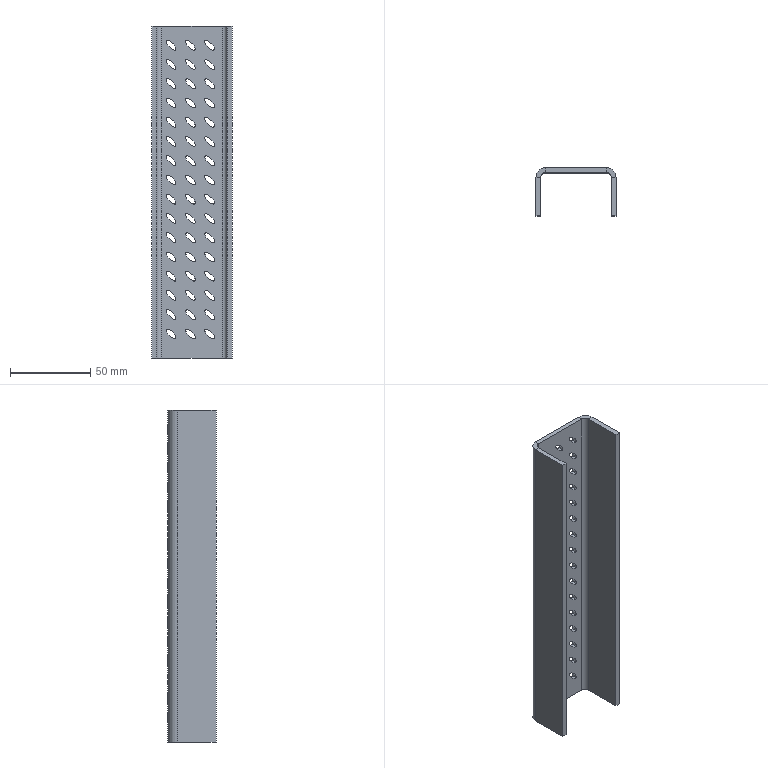Part | STEP file | SYL_0392D6J1SYL0380DJ10-1018359 | 1 solid | 118 faces | box 50 x 30 x 207 mm | volume 59466 mm3 | spline 96 | plane 18 | cylinder 4 | commonest cylinder face diameters 6 x2 12 x2